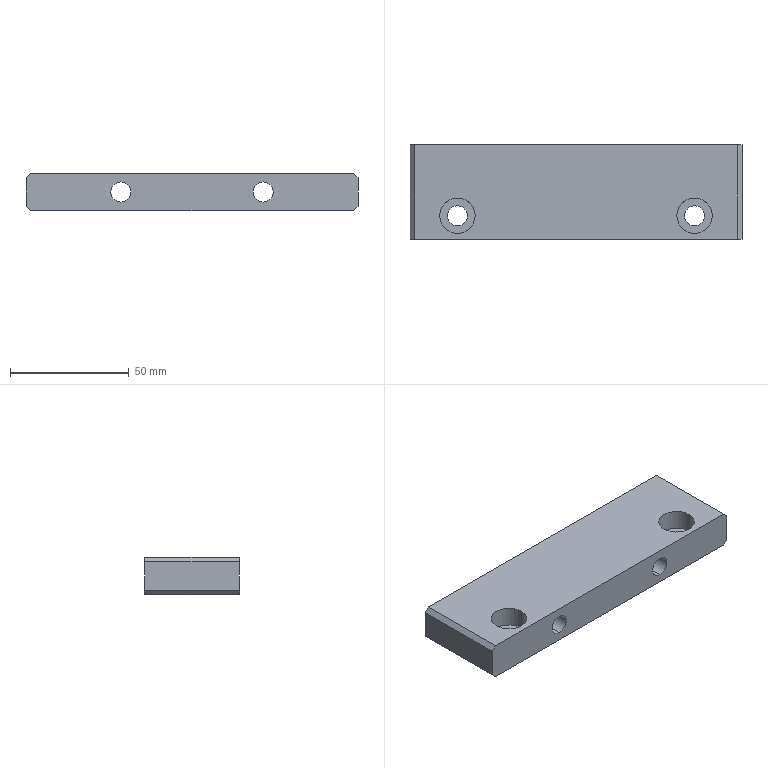Part | SolidWorks | features HoleWzd 2, Chamfer 1, Extrusion 1 | 1 solid | 24 faces | box 140 x 40 x 16 mm | volume 80881 mm3 | cylinder 12 | plane 12 | commonest cylinder face diameters 8.4 x4 8.5 x4 15 x4
STEP:
#1=CARTESIAN_POINT('',(12.5,10.,7.4));
#2=VERTEX_POINT('',#1);
#3=CARTESIAN_POINT('',(27.5,10.,7.4));
#4=VERTEX_POINT('',#3);
#5=CARTESIAN_POINT('',(20.,10.,7.4));
#6=DIRECTION('',(0.,0.,1.));
#7=DIRECTION('',(1.,0.,0.));
#8=AXIS2_PLACEMENT_3D('',#5,#6,#7);
#9=CIRCLE('',#8,7.5);
#10=EDGE_CURVE('',#2,#4,#9,.T.);
#11=ORIENTED_EDGE('',*,*,#10,.F.);
#12=CARTESIAN_POINT('',(12.5,10.,16.));
#13=VERTEX_POINT('',#12);
#14=CARTESIAN_POINT('',(12.5,10.,16.));
#15=DIRECTION('',(0.,0.,1.));
#16=VECTOR('',#15,1000.);
#17=LINE('',#14,#16);
#18=EDGE_CURVE('',#2,#13,#17,.T.);
#19=ORIENTED_EDGE('',*,*,#18,.T.);
#20=CARTESIAN_POINT('',(27.5,10.,16.));
#21=VERTEX_POINT('',#20);
#22=CARTESIAN_POINT('',(20.,10.,16.));
#23=DIRECTION('',(0.,0.,1.));
#24=DIRECTION('',(1.,0.,0.));
#25=AXIS2_PLACEMENT_3D('',#22,#23,#24);
#26=CIRCLE('',#25,7.5);
#27=EDGE_CURVE('',#13,#21,#26,.T.);
#28=ORIENTED_EDGE('',*,*,#27,.T.);
#29=CARTESIAN_POINT('',(27.5,10.,16.));
#30=DIRECTION('',(0.,0.,1.));
#31=VECTOR('',#30,1000.);
#32=LINE('',#29,#31);
#33=EDGE_CURVE('',#4,#21,#32,.T.);
#34=ORIENTED_EDGE('',*,*,#33,.F.);
#35=EDGE_LOOP('',(#11,#19,#28,#34));
#36=FACE_OUTER_BOUND('',#35,.T.);
#37=CARTESIAN_POINT('',(20.,10.,16.));
#38=DIRECTION('',(0.,0.,1.));
#39=DIRECTION('',(1.,0.,0.));
#40=AXIS2_PLACEMENT_3D('',#37,#38,#39);
#41=CYLINDRICAL_SURFACE('',#40,7.5);
#42=ADVANCED_FACE('',(#36),#41,.F.);
#43=CARTESIAN_POINT('',(15.8,10.,0.));
#44=VERTEX_POINT('',#43);
#45=CARTESIAN_POINT('',(24.2,10.,0.));
#46=VERTEX_POINT('',#45);
#47=CARTESIAN_POINT('',(20.,10.,0.));
#48=DIRECTION('',(0.,0.,1.));
#49=DIRECTION('',(1.,0.,0.));
#50=AXIS2_PLACEMENT_3D('',#47,#48,#49);
#51=CIRCLE('',#50,4.2);
#52=EDGE_CURVE('',#44,#46,#51,.T.);
#53=ORIENTED_EDGE('',*,*,#52,.F.);
#54=CARTESIAN_POINT('',(15.8,10.,7.4));
#55=VERTEX_POINT('',#54);
#56=CARTESIAN_POINT('',(15.8,10.,16.));
#57=DIRECTION('',(0.,0.,1.));
#58=VECTOR('',#57,1000.);
#59=LINE('',#56,#58);
#60=EDGE_CURVE('',#44,#55,#59,.T.);
#61=ORIENTED_EDGE('',*,*,#60,.T.);
#62=CARTESIAN_POINT('',(24.2,10.,7.4));
#63=VERTEX_POINT('',#62);
#64=CARTESIAN_POINT('',(20.,10.,7.4));
#65=DIRECTION('',(0.,0.,1.));
#66=DIRECTION('',(1.,0.,0.));
#67=AXIS2_PLACEMENT_3D('',#64,#65,#66);
#68=CIRCLE('',#67,4.2);
#69=EDGE_CURVE('',#55,#63,#68,.T.);
#70=ORIENTED_EDGE('',*,*,#69,.T.);
#71=CARTESIAN_POINT('',(24.2,10.,16.));
#72=DIRECTION('',(0.,0.,1.));
#73=VECTOR('',#72,1000.);
#74=LINE('',#71,#73);
#75=EDGE_CURVE('',#46,#63,#74,.T.);
#76=ORIENTED_EDGE('',*,*,#75,.F.);
#77=EDGE_LOOP('',(#53,#61,#70,#76));
#78=FACE_OUTER_BOUND('',#77,.T.);
#79=CARTESIAN_POINT('',(20.,10.,16.));
#80=DIRECTION('',(0.,0.,1.));
#81=DIRECTION('',(1.,0.,0.));
#82=AXIS2_PLACEMENT_3D('',#79,#80,#81);
#83=CYLINDRICAL_SURFACE('',#82,4.2);
#84=ADVANCED_FACE('',(#78),#83,.F.);
#85=CARTESIAN_POINT('',(112.5,10.,7.4));
#86=VERTEX_POINT('',#85);
#87=CARTESIAN_POINT('',(127.5,10.,7.4));
#88=VERTEX_POINT('',#87);
#89=CARTESIAN_POINT('',(120.,10.,7.4));
#90=DIRECTION('',(0.,0.,1.));
#91=DIRECTION('',(1.,0.,0.));
#92=AXIS2_PLACEMENT_3D('',#89,#90,#91);
#93=CIRCLE('',#92,7.5);
#94=EDGE_CURVE('',#86,#88,#93,.T.);
#95=ORIENTED_EDGE('',*,*,#94,.F.);
#96=CARTESIAN_POINT('',(112.5,10.,16.));
#97=VERTEX_POINT('',#96);
#98=CARTESIAN_POINT('',(112.5,10.,16.));
#99=DIRECTION('',(0.,0.,1.));
#100=VECTOR('',#99,1000.);
#101=LINE('',#98,#100);
#102=EDGE_CURVE('',#86,#97,#101,.T.);
#103=ORIENTED_EDGE('',*,*,#102,.T.);
#104=CARTESIAN_POINT('',(127.5,10.,16.));
#105=VERTEX_POINT('',#104);
#106=CARTESIAN_POINT('',(120.,10.,16.));
#107=DIRECTION('',(0.,0.,1.));
#108=DIRECTION('',(1.,0.,0.));
#109=AXIS2_PLACEMENT_3D('',#106,#107,#108);
#110=CIRCLE('',#109,7.5);
#111=EDGE_CURVE('',#97,#105,#110,.T.);
#112=ORIENTED_EDGE('',*,*,#111,.T.);
#113=CARTESIAN_POINT('',(127.5,10.,16.));
#114=DIRECTION('',(0.,0.,1.));
#115=VECTOR('',#114,1000.);
#116=LINE('',#113,#115);
#117=EDGE_CURVE('',#88,#105,#116,.T.);
#118=ORIENTED_EDGE('',*,*,#117,.F.);
#119=EDGE_LOOP('',(#95,#103,#112,#118));
#120=FACE_OUTER_BOUND('',#119,.T.);
#121=CARTESIAN_POINT('',(120.,10.,16.));
#122=DIRECTION('',(0.,0.,1.));
#123=DIRECTION('',(1.,0.,0.));
#124=AXIS2_PLACEMENT_3D('',#121,#122,#123);
#125=CYLINDRICAL_SURFACE('',#124,7.5);
#126=ADVANCED_FACE('',(#120),#125,.F.);
#127=CARTESIAN_POINT('',(115.8,10.,0.));
#128=VERTEX_POINT('',#127);
#129=CARTESIAN_POINT('',(124.2,10.,0.));
#130=VERTEX_POINT('',#129);
#131=CARTESIAN_POINT('',(120.,10.,0.));
#132=DIRECTION('',(0.,0.,1.));
#133=DIRECTION('',(1.,0.,0.));
#134=AXIS2_PLACEMENT_3D('',#131,#132,#133);
#135=CIRCLE('',#134,4.2);
#136=EDGE_CURVE('',#128,#130,#135,.T.);
#137=ORIENTED_EDGE('',*,*,#136,.F.);
#138=CARTESIAN_POINT('',(115.8,10.,7.4));
#139=VERTEX_POINT('',#138);
#140=CARTESIAN_POINT('',(115.8,10.,16.));
#141=DIRECTION('',(0.,0.,1.));
#142=VECTOR('',#141,1000.);
#143=LINE('',#140,#142);
#144=EDGE_CURVE('',#128,#139,#143,.T.);
#145=ORIENTED_EDGE('',*,*,#144,.T.);
#146=CARTESIAN_POINT('',(124.2,10.,7.4));
#147=VERTEX_POINT('',#146);
#148=CARTESIAN_POINT('',(120.,10.,7.4));
#149=DIRECTION('',(0.,0.,1.));
#150=DIRECTION('',(1.,0.,0.));
#151=AXIS2_PLACEMENT_3D('',#148,#149,#150);
#152=CIRCLE('',#151,4.2);
#153=EDGE_CURVE('',#139,#147,#152,.T.);
#154=ORIENTED_EDGE('',*,*,#153,.T.);
#155=CARTESIAN_POINT('',(124.2,10.,16.));
#156=DIRECTION('',(0.,0.,1.));
#157=VECTOR('',#156,1000.);
#158=LINE('',#155,#157);
#159=EDGE_CURVE('',#130,#147,#158,.T.);
#160=ORIENTED_EDGE('',*,*,#159,.F.);
#161=EDGE_LOOP('',(#137,#145,#154,#160));
#162=FACE_OUTER_BOUND('',#161,.T.);
#163=CARTESIAN_POINT('',(120.,10.,16.));
#164=DIRECTION('',(0.,0.,1.));
#165=DIRECTION('',(1.,0.,0.));
#166=AXIS2_PLACEMENT_3D('',#163,#164,#165);
#167=CYLINDRICAL_SURFACE('',#166,4.2);
#168=ADVANCED_FACE('',(#162),#167,.F.);
#169=CARTESIAN_POINT('',(40.,0.,3.75));
#170=VERTEX_POINT('',#169);
#171=CARTESIAN_POINT('',(40.,0.,12.25));
#172=VERTEX_POINT('',#171);
#173=CARTESIAN_POINT('',(40.,0.,8.));
#174=DIRECTION('',(0.,1.,0.));
#175=DIRECTION('',(0.,0.,1.));
#176=AXIS2_PLACEMENT_3D('',#173,#174,#175);
#177=CIRCLE('',#176,4.25);
#178=EDGE_CURVE('',#170,#172,#177,.T.);
#179=ORIENTED_EDGE('',*,*,#178,.F.);
#180=CARTESIAN_POINT('',(40.,40.,3.75));
#181=VERTEX_POINT('',#180);
#182=CARTESIAN_POINT('',(40.,40.,3.75));
#183=DIRECTION('',(0.,1.,0.));
#184=VECTOR('',#183,1000.);
#185=LINE('',#182,#184);
#186=EDGE_CURVE('',#170,#181,#185,.T.);
#187=ORIENTED_EDGE('',*,*,#186,.T.);
#188=CARTESIAN_POINT('',(40.,40.,12.25));
#189=VERTEX_POINT('',#188);
#190=CARTESIAN_POINT('',(40.,40.,8.));
#191=DIRECTION('',(0.,1.,0.));
#192=DIRECTION('',(0.,0.,1.));
#193=AXIS2_PLACEMENT_3D('',#190,#191,#192);
#194=CIRCLE('',#193,4.25);
#195=EDGE_CURVE('',#181,#189,#194,.T.);
#196=ORIENTED_EDGE('',*,*,#195,.T.);
#197=CARTESIAN_POINT('',(40.,40.,12.25));
#198=DIRECTION('',(0.,1.,0.));
#199=VECTOR('',#198,1000.);
#200=LINE('',#197,#199);
#201=EDGE_CURVE('',#172,#189,#200,.T.);
#202=ORIENTED_EDGE('',*,*,#201,.F.);
#203=EDGE_LOOP('',(#179,#187,#196,#202));
#204=FACE_OUTER_BOUND('',#203,.T.);
#205=CARTESIAN_POINT('',(40.,40.,8.));
#206=DIRECTION('',(0.,1.,0.));
#207=DIRECTION('',(0.,0.,1.));
#208=AXIS2_PLACEMENT_3D('',#205,#206,#207);
#209=CYLINDRICAL_SURFACE('',#208,4.25);
#210=ADVANCED_FACE('',(#204),#209,.F.);
#211=CARTESIAN_POINT('',(100.,0.,3.75));
#212=VERTEX_POINT('',#211);
#213=CARTESIAN_POINT('',(100.,0.,12.25));
#214=VERTEX_POINT('',#213);
#215=CARTESIAN_POINT('',(100.,0.,8.));
#216=DIRECTION('',(0.,1.,0.));
#217=DIRECTION('',(0.,0.,1.));
#218=AXIS2_PLACEMENT_3D('',#215,#216,#217);
#219=CIRCLE('',#218,4.25);
#220=EDGE_CURVE('',#212,#214,#219,.T.);
#221=ORIENTED_EDGE('',*,*,#220,.F.);
#222=CARTESIAN_POINT('',(100.,40.,3.75));
#223=VERTEX_POINT('',#222);
#224=CARTESIAN_POINT('',(100.,40.,3.75));
#225=DIRECTION('',(0.,1.,0.));
#226=VECTOR('',#225,1000.);
#227=LINE('',#224,#226);
#228=EDGE_CURVE('',#212,#223,#227,.T.);
#229=ORIENTED_EDGE('',*,*,#228,.T.);
#230=CARTESIAN_POINT('',(100.,40.,12.25));
#231=VERTEX_POINT('',#230);
#232=CARTESIAN_POINT('',(100.,40.,8.));
#233=DIRECTION('',(0.,1.,0.));
#234=DIRECTION('',(0.,0.,1.));
#235=AXIS2_PLACEMENT_3D('',#232,#233,#234);
#236=CIRCLE('',#235,4.25);
#237=EDGE_CURVE('',#223,#231,#236,.T.);
#238=ORIENTED_EDGE('',*,*,#237,.T.);
#239=CARTESIAN_POINT('',(100.,40.,12.25));
#240=DIRECTION('',(0.,1.,0.));
#241=VECTOR('',#240,1000.);
#242=LINE('',#239,#241);
#243=EDGE_CURVE('',#214,#231,#242,.T.);
#244=ORIENTED_EDGE('',*,*,#243,.F.);
#245=EDGE_LOOP('',(#221,#229,#238,#244));
#246=FACE_OUTER_BOUND('',#245,.T.);
#247=CARTESIAN_POINT('',(100.,40.,8.));
#248=DIRECTION('',(0.,1.,0.));
#249=DIRECTION('',(0.,0.,1.));
#250=AXIS2_PLACEMENT_3D('',#247,#248,#249);
#251=CYLINDRICAL_SURFACE('',#250,4.25);
#252=ADVANCED_FACE('',(#246),#251,.F.);
#253=CARTESIAN_POINT('',(0.,0.,14.));
#254=VERTEX_POINT('',#253);
#255=CARTESIAN_POINT('',(0.,0.,2.));
#256=VERTEX_POINT('',#255);
#257=CARTESIAN_POINT('',(0.,0.,16.));
#258=DIRECTION('',(0.,0.,-1.));
#259=VECTOR('',#258,1000.);
#260=LINE('',#257,#259);
#261=EDGE_CURVE('',#254,#256,#260,.T.);
#262=ORIENTED_EDGE('',*,*,#261,.F.);
#263=CARTESIAN_POINT('',(0.,40.,14.));
#264=VERTEX_POINT('',#263);
#265=CARTESIAN_POINT('',(0.,0.,14.));
#266=DIRECTION('',(0.,1.,0.));
#267=VECTOR('',#266,1000.);
#268=LINE('',#265,#267);
#269=EDGE_CURVE('',#254,#264,#268,.T.);
#270=ORIENTED_EDGE('',*,*,#269,.T.);
#271=CARTESIAN_POINT('',(0.,40.,2.));
#272=VERTEX_POINT('',#271);
#273=CARTESIAN_POINT('',(0.,40.,16.));
#274=DIRECTION('',(0.,0.,-1.));
#275=VECTOR('',#274,1000.);
#276=LINE('',#273,#275);
#277=EDGE_CURVE('',#264,#272,#276,.T.);
#278=ORIENTED_EDGE('',*,*,#277,.T.);
#279=CARTESIAN_POINT('',(0.,0.,2.));
#280=DIRECTION('',(0.,-1.,0.));
#281=VECTOR('',#280,1000.);
#282=LINE('',#279,#281);
#283=EDGE_CURVE('',#272,#256,#282,.T.);
#284=ORIENTED_EDGE('',*,*,#283,.T.);
#285=EDGE_LOOP('',(#262,#270,#278,#284));
#286=FACE_OUTER_BOUND('',#285,.T.);
#287=CARTESIAN_POINT('',(0.,0.,16.));
#288=DIRECTION('',(1.,0.,0.));
#289=DIRECTION('',(0.,0.,-1.));
#290=AXIS2_PLACEMENT_3D('',#287,#288,#289);
#291=PLANE('',#290);
#292=ADVANCED_FACE('',(#286),#291,.F.);
#293=CARTESIAN_POINT('',(40.,0.,8.));
#294=DIRECTION('',(0.,1.,0.));
#295=DIRECTION('',(0.,0.,1.));
#296=AXIS2_PLACEMENT_3D('',#293,#294,#295);
#297=CIRCLE('',#296,4.25);
#298=EDGE_CURVE('',#172,#170,#297,.T.);
#299=ORIENTED_EDGE('',*,*,#298,.T.);
#300=ORIENTED_EDGE('',*,*,#178,.T.);
#301=EDGE_LOOP('',(#299,#300));
#302=FACE_BOUND('',#301,.T.);
#303=CARTESIAN_POINT('',(100.,0.,8.));
#304=DIRECTION('',(0.,1.,0.));
#305=DIRECTION('',(0.,0.,1.));
#306=AXIS2_PLACEMENT_3D('',#303,#304,#305);
#307=CIRCLE('',#306,4.25);
#308=EDGE_CURVE('',#214,#212,#307,.T.);
#309=ORIENTED_EDGE('',*,*,#308,.T.);
#310=ORIENTED_EDGE('',*,*,#220,.T.);
#311=EDGE_LOOP('',(#309,#310));
#312=FACE_BOUND('',#311,.T.);
#313=CARTESIAN_POINT('',(140.,0.,14.));
#314=VERTEX_POINT('',#313);
#315=CARTESIAN_POINT('',(140.,0.,2.));
#316=VERTEX_POINT('',#315);
#317=CARTESIAN_POINT('',(140.,0.,16.));
#318=DIRECTION('',(0.,0.,-1.));
#319=VECTOR('',#318,1000.);
#320=LINE('',#317,#319);
#321=EDGE_CURVE('',#314,#316,#320,.T.);
#322=ORIENTED_EDGE('',*,*,#321,.F.);
#323=CARTESIAN_POINT('',(138.,0.,16.));
#324=VERTEX_POINT('',#323);
#325=CARTESIAN_POINT('',(138.,0.,16.));
#326=DIRECTION('',(-0.7071,0.,0.7071));
#327=VECTOR('',#326,1000.);
#328=LINE('',#325,#327);
#329=EDGE_CURVE('',#314,#324,#328,.T.);
#330=ORIENTED_EDGE('',*,*,#329,.T.);
#331=CARTESIAN_POINT('',(2.,0.,16.));
#332=VERTEX_POINT('',#331);
#333=CARTESIAN_POINT('',(0.,0.,16.));
#334=DIRECTION('',(1.,0.,0.));
#335=VECTOR('',#334,1000.);
#336=LINE('',#333,#335);
#337=EDGE_CURVE('',#332,#324,#336,.T.);
#338=ORIENTED_EDGE('',*,*,#337,.F.);
#339=CARTESIAN_POINT('',(2.,0.,16.));
#340=DIRECTION('',(-0.7071,0.,-0.7071));
#341=VECTOR('',#340,1000.);
#342=LINE('',#339,#341);
#343=EDGE_CURVE('',#332,#254,#342,.T.);
#344=ORIENTED_EDGE('',*,*,#343,.T.);
#345=ORIENTED_EDGE('',*,*,#261,.T.);
#346=CARTESIAN_POINT('',(2.,0.,0.));
#347=VERTEX_POINT('',#346);
#348=CARTESIAN_POINT('',(0.,0.,2.));
#349=DIRECTION('',(0.7071,0.,-0.7071));
#350=VECTOR('',#349,1000.);
#351=LINE('',#348,#350);
#352=EDGE_CURVE('',#256,#347,#351,.T.);
#353=ORIENTED_EDGE('',*,*,#352,.T.);
#354=CARTESIAN_POINT('',(138.,0.,0.));
#355=VERTEX_POINT('',#354);
#356=CARTESIAN_POINT('',(0.,0.,0.));
#357=DIRECTION('',(1.,0.,0.));
#358=VECTOR('',#357,1000.);
#359=LINE('',#356,#358);
#360=EDGE_CURVE('',#347,#355,#359,.T.);
#361=ORIENTED_EDGE('',*,*,#360,.T.);
#362=CARTESIAN_POINT('',(140.,0.,2.));
#363=DIRECTION('',(0.7071,0.,0.7071));
#364=VECTOR('',#363,1000.);
#365=LINE('',#362,#364);
#366=EDGE_CURVE('',#355,#316,#365,.T.);
#367=ORIENTED_EDGE('',*,*,#366,.T.);
#368=EDGE_LOOP('',(#322,#330,#338,#344,#345,#353,#361,#367));
#369=FACE_OUTER_BOUND('',#368,.T.);
#370=CARTESIAN_POINT('',(0.,0.,16.));
#371=DIRECTION('',(0.,1.,0.));
#372=DIRECTION('',(0.,0.,1.));
#373=AXIS2_PLACEMENT_3D('',#370,#371,#372);
#374=PLANE('',#373);
#375=ADVANCED_FACE('',(#302,#312,#369),#374,.F.);
#376=CARTESIAN_POINT('',(140.,40.,14.));
#377=VERTEX_POINT('',#376);
#378=CARTESIAN_POINT('',(140.,40.,2.));
#379=VERTEX_POINT('',#378);
#380=CARTESIAN_POINT('',(140.,40.,16.));
#381=DIRECTION('',(0.,0.,-1.));
#382=VECTOR('',#381,1000.);
#383=LINE('',#380,#382);
#384=EDGE_CURVE('',#377,#379,#383,.T.);
#385=ORIENTED_EDGE('',*,*,#384,.F.);
#386=CARTESIAN_POINT('',(140.,0.,14.));
#387=DIRECTION('',(0.,-1.,0.));
#388=VECTOR('',#387,1000.);
#389=LINE('',#386,#388);
#390=EDGE_CURVE('',#377,#314,#389,.T.);
#391=ORIENTED_EDGE('',*,*,#390,.T.);
#392=ORIENTED_EDGE('',*,*,#321,.T.);
#393=CARTESIAN_POINT('',(140.,40.,2.));
#394=DIRECTION('',(0.,1.,0.));
#395=VECTOR('',#394,1000.);
#396=LINE('',#393,#395);
#397=EDGE_CURVE('',#316,#379,#396,.T.);
#398=ORIENTED_EDGE('',*,*,#397,.T.);
#399=EDGE_LOOP('',(#385,#391,#392,#398));
#400=FACE_OUTER_BOUND('',#399,.T.);
#401=CARTESIAN_POINT('',(140.,0.,16.));
#402=DIRECTION('',(-1.,0.,0.));
#403=DIRECTION('',(0.,0.,1.));
#404=AXIS2_PLACEMENT_3D('',#401,#402,#403);
#405=PLANE('',#404);
#406=ADVANCED_FACE('',(#400),#405,.F.);
#407=CARTESIAN_POINT('',(40.,40.,8.));
#408=DIRECTION('',(0.,1.,0.));
#409=DIRECTION('',(0.,0.,1.));
#410=AXIS2_PLACEMENT_3D('',#407,#408,#409);
#411=CIRCLE('',#410,4.25);
#412=EDGE_CURVE('',#189,#181,#411,.T.);
#413=ORIENTED_EDGE('',*,*,#412,.F.);
#414=ORIENTED_EDGE('',*,*,#195,.F.);
#415=EDGE_LOOP('',(#413,#414));
#416=FACE_BOUND('',#415,.T.);
#417=CARTESIAN_POINT('',(100.,40.,8.));
#418=DIRECTION('',(0.,1.,0.));
#419=DIRECTION('',(0.,0.,1.));
#420=AXIS2_PLACEMENT_3D('',#417,#418,#419);
#421=CIRCLE('',#420,4.25);
#422=EDGE_CURVE('',#231,#223,#421,.T.);
#423=ORIENTED_EDGE('',*,*,#422,.F.);
#424=ORIENTED_EDGE('',*,*,#237,.F.);
#425=EDGE_LOOP('',(#423,#424));
#426=FACE_BOUND('',#425,.T.);
#427=CARTESIAN_POINT('',(138.,40.,16.));
#428=VERTEX_POINT('',#427);
#429=CARTESIAN_POINT('',(2.,40.,16.));
#430=VERTEX_POINT('',#429);
#431=CARTESIAN_POINT('',(0.,40.,16.));
#432=DIRECTION('',(-1.,0.,0.));
#433=VECTOR('',#432,1000.);
#434=LINE('',#431,#433);
#435=EDGE_CURVE('',#428,#430,#434,.T.);
#436=ORIENTED_EDGE('',*,*,#435,.F.);
#437=CARTESIAN_POINT('',(138.,40.,16.));
#438=DIRECTION('',(0.7071,0.,-0.7071));
#439=VECTOR('',#438,1000.);
#440=LINE('',#437,#439);
#441=EDGE_CURVE('',#428,#377,#440,.T.);
#442=ORIENTED_EDGE('',*,*,#441,.T.);
#443=ORIENTED_EDGE('',*,*,#384,.T.);
#444=CARTESIAN_POINT('',(138.,40.,0.));
#445=VERTEX_POINT('',#444);
#446=CARTESIAN_POINT('',(140.,40.,2.));
#447=DIRECTION('',(-0.7071,0.,-0.7071));
#448=VECTOR('',#447,1000.);
#449=LINE('',#446,#448);
#450=EDGE_CURVE('',#379,#445,#449,.T.);
#451=ORIENTED_EDGE('',*,*,#450,.T.);
#452=CARTESIAN_POINT('',(2.,40.,0.));
#453=VERTEX_POINT('',#452);
#454=CARTESIAN_POINT('',(0.,40.,0.));
#455=DIRECTION('',(-1.,0.,0.));
#456=VECTOR('',#455,1000.);
#457=LINE('',#454,#456);
#458=EDGE_CURVE('',#445,#453,#457,.T.);
#459=ORIENTED_EDGE('',*,*,#458,.T.);
#460=CARTESIAN_POINT('',(0.,40.,2.));
#461=DIRECTION('',(-0.7071,0.,0.7071));
#462=VECTOR('',#461,1000.);
#463=LINE('',#460,#462);
#464=EDGE_CURVE('',#453,#272,#463,.T.);
#465=ORIENTED_EDGE('',*,*,#464,.T.);
#466=ORIENTED_EDGE('',*,*,#277,.F.);
#467=CARTESIAN_POINT('',(2.,40.,16.));
#468=DIRECTION('',(0.7071,0.,0.7071));
#469=VECTOR('',#468,1000.);
#470=LINE('',#467,#469);
#471=EDGE_CURVE('',#264,#430,#470,.T.);
#472=ORIENTED_EDGE('',*,*,#471,.T.);
#473=EDGE_LOOP('',(#436,#442,#443,#451,#459,#465,#466,#472));
#474=FACE_OUTER_BOUND('',#473,.T.);
#475=CARTESIAN_POINT('',(0.,40.,16.));
#476=DIRECTION('',(0.,-1.,0.));
#477=DIRECTION('',(0.,0.,-1.));
#478=AXIS2_PLACEMENT_3D('',#475,#476,#477);
#479=PLANE('',#478);
#480=ADVANCED_FACE('',(#416,#426,#474),#479,.F.);
#481=CARTESIAN_POINT('',(20.,10.,16.));
#482=DIRECTION('',(0.,0.,1.));
#483=DIRECTION('',(1.,0.,0.));
#484=AXIS2_PLACEMENT_3D('',#481,#482,#483);
#485=CIRCLE('',#484,7.5);
#486=EDGE_CURVE('',#21,#13,#485,.T.);
#487=ORIENTED_EDGE('',*,*,#486,.F.);
#488=ORIENTED_EDGE('',*,*,#27,.F.);
#489=EDGE_LOOP('',(#487,#488));
#490=FACE_BOUND('',#489,.T.);
#491=CARTESIAN_POINT('',(120.,10.,16.));
#492=DIRECTION('',(0.,0.,1.));
#493=DIRECTION('',(1.,0.,0.));
#494=AXIS2_PLACEMENT_3D('',#491,#492,#493);
#495=CIRCLE('',#494,7.5);
#496=EDGE_CURVE('',#105,#97,#495,.T.);
#497=ORIENTED_EDGE('',*,*,#496,.F.);
#498=ORIENTED_EDGE('',*,*,#111,.F.);
#499=EDGE_LOOP('',(#497,#498));
#500=FACE_BOUND('',#499,.T.);
#501=ORIENTED_EDGE('',*,*,#337,.T.);
#502=CARTESIAN_POINT('',(138.,0.,16.));
#503=DIRECTION('',(0.,1.,0.));
#504=VECTOR('',#503,1000.);
#505=LINE('',#502,#504);
#506=EDGE_CURVE('',#324,#428,#505,.T.);
#507=ORIENTED_EDGE('',*,*,#506,.T.);
#508=ORIENTED_EDGE('',*,*,#435,.T.);
#509=CARTESIAN_POINT('',(2.,0.,16.));
#510=DIRECTION('',(0.,-1.,0.));
#511=VECTOR('',#510,1000.);
#512=LINE('',#509,#511);
#513=EDGE_CURVE('',#430,#332,#512,.T.);
#514=ORIENTED_EDGE('',*,*,#513,.T.);
#515=EDGE_LOOP('',(#501,#507,#508,#514));
#516=FACE_OUTER_BOUND('',#515,.T.);
#517=CARTESIAN_POINT('',(0.,0.,16.));
#518=DIRECTION('',(0.,0.,-1.));
#519=DIRECTION('',(-1.,0.,0.));
#520=AXIS2_PLACEMENT_3D('',#517,#518,#519);
#521=PLANE('',#520);
#522=ADVANCED_FACE('',(#490,#500,#516),#521,.F.);
#523=CARTESIAN_POINT('',(20.,10.,0.));
#524=DIRECTION('',(0.,0.,1.));
#525=DIRECTION('',(1.,0.,0.));
#526=AXIS2_PLACEMENT_3D('',#523,#524,#525);
#527=CIRCLE('',#526,4.2);
#528=EDGE_CURVE('',#46,#44,#527,.T.);
#529=ORIENTED_EDGE('',*,*,#528,.T.);
#530=ORIENTED_EDGE('',*,*,#52,.T.);
#531=EDGE_LOOP('',(#529,#530));
#532=FACE_BOUND('',#531,.T.);
#533=CARTESIAN_POINT('',(120.,10.,0.));
#534=DIRECTION('',(0.,0.,1.));
#535=DIRECTION('',(1.,0.,0.));
#536=AXIS2_PLACEMENT_3D('',#533,#534,#535);
#537=CIRCLE('',#536,4.2);
#538=EDGE_CURVE('',#130,#128,#537,.T.);
#539=ORIENTED_EDGE('',*,*,#538,.T.);
#540=ORIENTED_EDGE('',*,*,#136,.T.);
#541=EDGE_LOOP('',(#539,#540));
#542=FACE_BOUND('',#541,.T.);
#543=ORIENTED_EDGE('',*,*,#360,.F.);
#544=CARTESIAN_POINT('',(2.,40.,0.));
#545=DIRECTION('',(0.,1.,0.));
#546=VECTOR('',#545,1000.);
#547=LINE('',#544,#546);
#548=EDGE_CURVE('',#347,#453,#547,.T.);
#549=ORIENTED_EDGE('',*,*,#548,.T.);
#550=ORIENTED_EDGE('',*,*,#458,.F.);
#551=CARTESIAN_POINT('',(138.,0.,0.));
#552=DIRECTION('',(0.,-1.,0.));
#553=VECTOR('',#552,1000.);
#554=LINE('',#551,#553);
#555=EDGE_CURVE('',#445,#355,#554,.T.);
#556=ORIENTED_EDGE('',*,*,#555,.T.);
#557=EDGE_LOOP('',(#543,#549,#550,#556));
#558=FACE_OUTER_BOUND('',#557,.T.);
#559=CARTESIAN_POINT('',(0.,0.,0.));
#560=DIRECTION('',(0.,0.,-1.));
#561=DIRECTION('',(-1.,0.,0.));
#562=AXIS2_PLACEMENT_3D('',#559,#560,#561);
#563=PLANE('',#562);
#564=ADVANCED_FACE('',(#532,#542,#558),#563,.T.);
#565=ORIENTED_EDGE('',*,*,#228,.F.);
#566=ORIENTED_EDGE('',*,*,#308,.F.);
#567=ORIENTED_EDGE('',*,*,#243,.T.);
#568=ORIENTED_EDGE('',*,*,#422,.T.);
#569=EDGE_LOOP('',(#565,#566,#567,#568));
#570=FACE_OUTER_BOUND('',#569,.T.);
#571=CARTESIAN_POINT('',(100.,40.,8.));
#572=DIRECTION('',(0.,1.,0.));
#573=DIRECTION('',(0.,0.,1.));
#574=AXIS2_PLACEMENT_3D('',#571,#572,#573);
#575=CYLINDRICAL_SURFACE('',#574,4.25);
#576=ADVANCED_FACE('',(#570),#575,.F.);
#577=ORIENTED_EDGE('',*,*,#186,.F.);
#578=ORIENTED_EDGE('',*,*,#298,.F.);
#579=ORIENTED_EDGE('',*,*,#201,.T.);
#580=ORIENTED_EDGE('',*,*,#412,.T.);
#581=EDGE_LOOP('',(#577,#578,#579,#580));
#582=FACE_OUTER_BOUND('',#581,.T.);
#583=CARTESIAN_POINT('',(40.,40.,8.));
#584=DIRECTION('',(0.,1.,0.));
#585=DIRECTION('',(0.,0.,1.));
#586=AXIS2_PLACEMENT_3D('',#583,#584,#585);
#587=CYLINDRICAL_SURFACE('',#586,4.25);
#588=ADVANCED_FACE('',(#582),#587,.F.);
#589=ORIENTED_EDGE('',*,*,#144,.F.);
#590=ORIENTED_EDGE('',*,*,#538,.F.);
#591=ORIENTED_EDGE('',*,*,#159,.T.);
#592=CARTESIAN_POINT('',(120.,10.,7.4));
#593=DIRECTION('',(0.,0.,1.));
#594=DIRECTION('',(1.,0.,0.));
#595=AXIS2_PLACEMENT_3D('',#592,#593,#594);
#596=CIRCLE('',#595,4.2);
#597=EDGE_CURVE('',#147,#139,#596,.T.);
#598=ORIENTED_EDGE('',*,*,#597,.T.);
#599=EDGE_LOOP('',(#589,#590,#591,#598));
#600=FACE_OUTER_BOUND('',#599,.T.);
#601=CARTESIAN_POINT('',(120.,10.,16.));
#602=DIRECTION('',(0.,0.,1.));
#603=DIRECTION('',(1.,0.,0.));
#604=AXIS2_PLACEMENT_3D('',#601,#602,#603);
#605=CYLINDRICAL_SURFACE('',#604,4.2);
#606=ADVANCED_FACE('',(#600),#605,.F.);
#607=ORIENTED_EDGE('',*,*,#597,.F.);
#608=ORIENTED_EDGE('',*,*,#153,.F.);
#609=EDGE_LOOP('',(#607,#608));
#610=FACE_BOUND('',#609,.T.);
#611=CARTESIAN_POINT('',(120.,10.,7.4));
#612=DIRECTION('',(0.,0.,1.));
#613=DIRECTION('',(1.,0.,0.));
#614=AXIS2_PLACEMENT_3D('',#611,#612,#613);
#615=CIRCLE('',#614,7.5);
#616=EDGE_CURVE('',#88,#86,#615,.T.);
#617=ORIENTED_EDGE('',*,*,#616,.T.);
#618=ORIENTED_EDGE('',*,*,#94,.T.);
#619=EDGE_LOOP('',(#617,#618));
#620=FACE_OUTER_BOUND('',#619,.T.);
#621=CARTESIAN_POINT('',(124.2,10.,7.4));
#622=DIRECTION('',(0.,0.,-1.));
#623=DIRECTION('',(-1.,0.,0.));
#624=AXIS2_PLACEMENT_3D('',#621,#622,#623);
#625=PLANE('',#624);
#626=ADVANCED_FACE('',(#610,#620),#625,.F.);
#627=ORIENTED_EDGE('',*,*,#102,.F.);
#628=ORIENTED_EDGE('',*,*,#616,.F.);
#629=ORIENTED_EDGE('',*,*,#117,.T.);
#630=ORIENTED_EDGE('',*,*,#496,.T.);
#631=EDGE_LOOP('',(#627,#628,#629,#630));
#632=FACE_OUTER_BOUND('',#631,.T.);
#633=CARTESIAN_POINT('',(120.,10.,16.));
#634=DIRECTION('',(0.,0.,1.));
#635=DIRECTION('',(1.,0.,0.));
#636=AXIS2_PLACEMENT_3D('',#633,#634,#635);
#637=CYLINDRICAL_SURFACE('',#636,7.5);
#638=ADVANCED_FACE('',(#632),#637,.F.);
#639=ORIENTED_EDGE('',*,*,#60,.F.);
#640=ORIENTED_EDGE('',*,*,#528,.F.);
#641=ORIENTED_EDGE('',*,*,#75,.T.);
#642=CARTESIAN_POINT('',(20.,10.,7.4));
#643=DIRECTION('',(0.,0.,1.));
#644=DIRECTION('',(1.,0.,0.));
#645=AXIS2_PLACEMENT_3D('',#642,#643,#644);
#646=CIRCLE('',#645,4.2);
#647=EDGE_CURVE('',#63,#55,#646,.T.);
#648=ORIENTED_EDGE('',*,*,#647,.T.);
#649=EDGE_LOOP('',(#639,#640,#641,#648));
#650=FACE_OUTER_BOUND('',#649,.T.);
#651=CARTESIAN_POINT('',(20.,10.,16.));
#652=DIRECTION('',(0.,0.,1.));
#653=DIRECTION('',(1.,0.,0.));
#654=AXIS2_PLACEMENT_3D('',#651,#652,#653);
#655=CYLINDRICAL_SURFACE('',#654,4.2);
#656=ADVANCED_FACE('',(#650),#655,.F.);
#657=ORIENTED_EDGE('',*,*,#647,.F.);
#658=ORIENTED_EDGE('',*,*,#69,.F.);
#659=EDGE_LOOP('',(#657,#658));
#660=FACE_BOUND('',#659,.T.);
#661=CARTESIAN_POINT('',(20.,10.,7.4));
#662=DIRECTION('',(0.,0.,1.));
#663=DIRECTION('',(1.,0.,0.));
#664=AXIS2_PLACEMENT_3D('',#661,#662,#663);
#665=CIRCLE('',#664,7.5);
#666=EDGE_CURVE('',#4,#2,#665,.T.);
#667=ORIENTED_EDGE('',*,*,#666,.T.);
#668=ORIENTED_EDGE('',*,*,#10,.T.);
#669=EDGE_LOOP('',(#667,#668));
#670=FACE_OUTER_BOUND('',#669,.T.);
#671=CARTESIAN_POINT('',(24.2,10.,7.4));
#672=DIRECTION('',(0.,0.,-1.));
#673=DIRECTION('',(-1.,0.,0.));
#674=AXIS2_PLACEMENT_3D('',#671,#672,#673);
#675=PLANE('',#674);
#676=ADVANCED_FACE('',(#660,#670),#675,.F.);
#677=ORIENTED_EDGE('',*,*,#18,.F.);
#678=ORIENTED_EDGE('',*,*,#666,.F.);
#679=ORIENTED_EDGE('',*,*,#33,.T.);
#680=ORIENTED_EDGE('',*,*,#486,.T.);
#681=EDGE_LOOP('',(#677,#678,#679,#680));
#682=FACE_OUTER_BOUND('',#681,.T.);
#683=CARTESIAN_POINT('',(20.,10.,16.));
#684=DIRECTION('',(0.,0.,1.));
#685=DIRECTION('',(1.,0.,0.));
#686=AXIS2_PLACEMENT_3D('',#683,#684,#685);
#687=CYLINDRICAL_SURFACE('',#686,7.5);
#688=ADVANCED_FACE('',(#682),#687,.F.);
#689=ORIENTED_EDGE('',*,*,#329,.F.);
#690=ORIENTED_EDGE('',*,*,#390,.F.);
#691=ORIENTED_EDGE('',*,*,#441,.F.);
#692=ORIENTED_EDGE('',*,*,#506,.F.);
#693=EDGE_LOOP('',(#689,#690,#691,#692));
#694=FACE_OUTER_BOUND('',#693,.T.);
#695=CARTESIAN_POINT('',(138.,0.,16.));
#696=DIRECTION('',(-0.7071,0.,-0.7071));
#697=DIRECTION('',(0.,1.,0.));
#698=AXIS2_PLACEMENT_3D('',#695,#696,#697);
#699=PLANE('',#698);
#700=ADVANCED_FACE('',(#694),#699,.F.);
#701=ORIENTED_EDGE('',*,*,#471,.F.);
#702=ORIENTED_EDGE('',*,*,#269,.F.);
#703=ORIENTED_EDGE('',*,*,#343,.F.);
#704=ORIENTED_EDGE('',*,*,#513,.F.);
#705=EDGE_LOOP('',(#701,#702,#703,#704));
#706=FACE_OUTER_BOUND('',#705,.T.);
#707=CARTESIAN_POINT('',(2.,0.,16.));
#708=DIRECTION('',(0.7071,0.,-0.7071));
#709=DIRECTION('',(0.,-1.,0.));
#710=AXIS2_PLACEMENT_3D('',#707,#708,#709);
#711=PLANE('',#710);
#712=ADVANCED_FACE('',(#706),#711,.F.);
#713=ORIENTED_EDGE('',*,*,#464,.F.);
#714=ORIENTED_EDGE('',*,*,#548,.F.);
#715=ORIENTED_EDGE('',*,*,#352,.F.);
#716=ORIENTED_EDGE('',*,*,#283,.F.);
#717=EDGE_LOOP('',(#713,#714,#715,#716));
#718=FACE_OUTER_BOUND('',#717,.T.);
#719=CARTESIAN_POINT('',(0.,0.,2.));
#720=DIRECTION('',(-0.7071,0.,-0.7071));
#721=DIRECTION('',(0.,1.,0.));
#722=AXIS2_PLACEMENT_3D('',#719,#720,#721);
#723=PLANE('',#722);
#724=ADVANCED_FACE('',(#718),#723,.T.);
#725=ORIENTED_EDGE('',*,*,#366,.F.);
#726=ORIENTED_EDGE('',*,*,#555,.F.);
#727=ORIENTED_EDGE('',*,*,#450,.F.);
#728=ORIENTED_EDGE('',*,*,#397,.F.);
#729=EDGE_LOOP('',(#725,#726,#727,#728));
#730=FACE_OUTER_BOUND('',#729,.T.);
#731=CARTESIAN_POINT('',(140.,0.,2.));
#732=DIRECTION('',(0.7071,0.,-0.7071));
#733=DIRECTION('',(0.,-1.,0.));
#734=AXIS2_PLACEMENT_3D('',#731,#732,#733);
#735=PLANE('',#734);
#736=ADVANCED_FACE('',(#730),#735,.T.);
#737=CLOSED_SHELL('',(#42,#84,#126,#168,#210,#252,#292,#375,#406,#480,#522,#564,#576,#588,#606,#626,#638,#656,#676,#688,#700,#712,#724,#736));
#738=MANIFOLD_SOLID_BREP('',#737);
#739=CARTESIAN_POINT('',(0.,0.,0.));
#740=DIRECTION('',(0.,0.,1.));
#741=DIRECTION('',(1.,0.,0.));
#742=AXIS2_PLACEMENT_3D('',#739,#740,#741);
#743=(LENGTH_UNIT()NAMED_UNIT(*)SI_UNIT(.MILLI.,.METRE.));
#744=UNCERTAINTY_MEASURE_WITH_UNIT(LENGTH_MEASURE(0.00001),#743,'','');
#745=(NAMED_UNIT(*)PLANE_ANGLE_UNIT()SI_UNIT($,.RADIAN.));
#746=(NAMED_UNIT(*)SI_UNIT($,.STERADIAN.)SOLID_ANGLE_UNIT());
#747=(GEOMETRIC_REPRESENTATION_CONTEXT(3)GLOBAL_UNCERTAINTY_ASSIGNED_CONTEXT((#744))GLOBAL_UNIT_ASSIGNED_CONTEXT((#743,#745,#746))REPRESENTATION_CONTEXT('',''));
#748=ADVANCED_BREP_SHAPE_REPRESENTATION('',(#738,#742),#747);